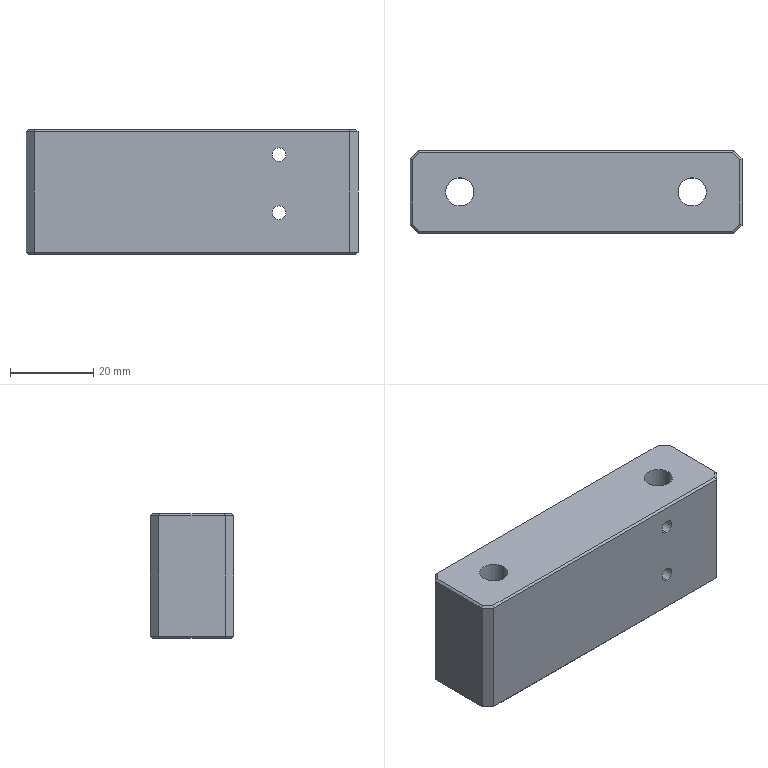Part | STEP file | PN_0002 motor pillar_Default | 1 solid | 34 faces | box 80 x 20 x 30 mm | volume 45190 mm3 | plane 26 | cylinder 8 | commonest cylinder face diameters 3.3 x4 6.8 x4